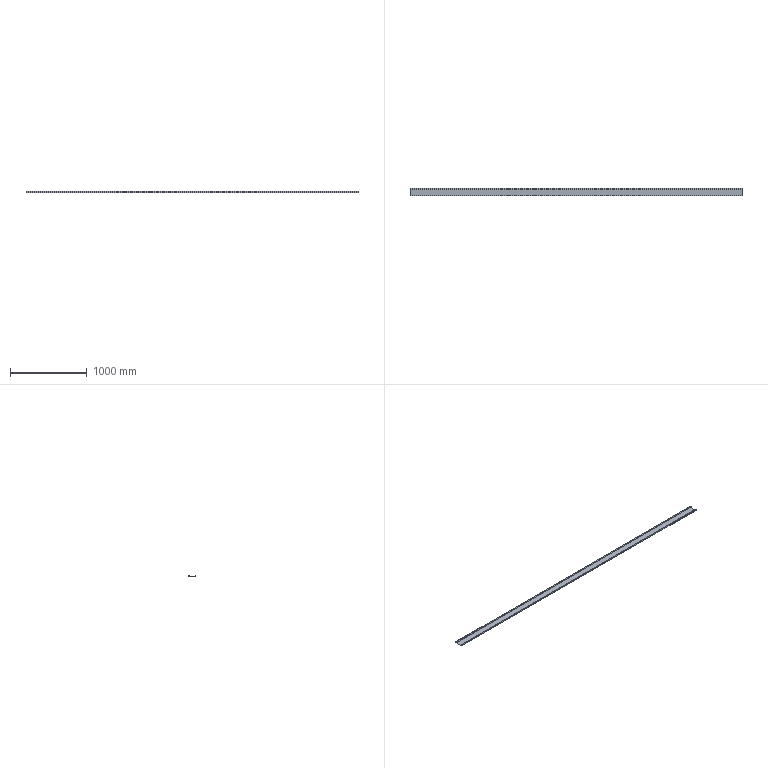Part | STEP file | 电柜护栏4踢脚Plate | 1 solid | 18 faces | box 4333 x 100 x 20 mm | volume 996027 mm3 | plane 12 | cylinder 6 | commonest cylinder face diameters 2 x3 5 x3
STEP:
#1=CARTESIAN_POINT('',(0.,0.,0.));
#2=DIRECTION('',(0.,0.,1.));
#3=DIRECTION('',(1.,0.,0.));
#4=AXIS2_PLACEMENT_3D('',#1,#2,#3);
#5=CARTESIAN_POINT('',(-2166.5,1.5,2.5));
#6=VERTEX_POINT('',#5);
#7=CARTESIAN_POINT('',(-2166.5,1.5,20.));
#8=VERTEX_POINT('',#7);
#9=CARTESIAN_POINT('',(-2166.5,1.5,2.5));
#10=DIRECTION('',(0.,0.,1.));
#11=VECTOR('',#10,1.);
#12=LINE('',#9,#11);
#13=CARTESIAN_POINT('',(2166.5,1.5,2.5));
#14=DIRECTION('',(0.,-1.,0.));
#15=DIRECTION('',(0.,0.,-1.));
#16=AXIS2_PLACEMENT_3D('',#13,#14,#15);
#17=PLANE('',#16);
#18=CARTESIAN_POINT('',(0.,-4333.));
#19=DIRECTION('',(-1.,0.));
#20=VECTOR('',#19,1.);
#21=LINE('',#18,#20);
#22=(GEOMETRIC_REPRESENTATION_CONTEXT(2)PARAMETRIC_REPRESENTATION_CONTEXT()REPRESENTATION_CONTEXT('',''));
#23=DEFINITIONAL_REPRESENTATION('',(#21),#22);
#24=PCURVE('',#17,#23);
#25=CARTESIAN_POINT('',(-2166.5,2.5,2.5));
#26=DIRECTION('',(-1.,0.,0.));
#27=DIRECTION('',(0.,0.,1.));
#28=AXIS2_PLACEMENT_3D('',#25,#26,#27);
#29=PLANE('',#28);
#30=CARTESIAN_POINT('',(0.,-1.));
#31=DIRECTION('',(1.,0.));
#32=VECTOR('',#31,1.);
#33=LINE('',#30,#32);
#34=(GEOMETRIC_REPRESENTATION_CONTEXT(2)PARAMETRIC_REPRESENTATION_CONTEXT()REPRESENTATION_CONTEXT('',''));
#35=DEFINITIONAL_REPRESENTATION('',(#33),#34);
#36=PCURVE('',#29,#35);
#37=SURFACE_CURVE('',#12,(#24,#36),.PCURVE_S1.);
#38=EDGE_CURVE('',#6,#8,#37,.T.);
#39=ORIENTED_EDGE('',*,*,#38,.T.);
#40=CARTESIAN_POINT('',(2166.5,1.5,20.));
#41=VERTEX_POINT('',#40);
#42=CARTESIAN_POINT('',(2166.5,1.5,20.));
#43=DIRECTION('',(-1.,0.,0.));
#44=VECTOR('',#43,1.);
#45=LINE('',#42,#44);
#46=CARTESIAN_POINT('',(-17.5,0.));
#47=DIRECTION('',(0.,-1.));
#48=VECTOR('',#47,1.);
#49=LINE('',#46,#48);
#50=(GEOMETRIC_REPRESENTATION_CONTEXT(2)PARAMETRIC_REPRESENTATION_CONTEXT()REPRESENTATION_CONTEXT('',''));
#51=DEFINITIONAL_REPRESENTATION('',(#49),#50);
#52=PCURVE('',#17,#51);
#53=CARTESIAN_POINT('',(2166.5,0.,20.));
#54=DIRECTION('',(0.,0.,1.));
#55=DIRECTION('',(1.,0.,0.));
#56=AXIS2_PLACEMENT_3D('',#53,#54,#55);
#57=PLANE('',#56);
#58=CARTESIAN_POINT('',(0.,1.5));
#59=DIRECTION('',(-1.,0.));
#60=VECTOR('',#59,1.);
#61=LINE('',#58,#60);
#62=(GEOMETRIC_REPRESENTATION_CONTEXT(2)PARAMETRIC_REPRESENTATION_CONTEXT()REPRESENTATION_CONTEXT('',''));
#63=DEFINITIONAL_REPRESENTATION('',(#61),#62);
#64=PCURVE('',#57,#63);
#65=SURFACE_CURVE('',#45,(#52,#64),.PCURVE_S1.);
#66=EDGE_CURVE('',#41,#8,#65,.T.);
#67=ORIENTED_EDGE('',*,*,#66,.F.);
#68=CARTESIAN_POINT('',(2166.5,1.5,2.5));
#69=VERTEX_POINT('',#68);
#70=CARTESIAN_POINT('',(2166.5,1.5,2.5));
#71=DIRECTION('',(0.,0.,1.));
#72=VECTOR('',#71,1.);
#73=LINE('',#70,#72);
#74=CARTESIAN_POINT('',(0.,0.));
#75=DIRECTION('',(-1.,0.));
#76=VECTOR('',#75,1.);
#77=LINE('',#74,#76);
#78=(GEOMETRIC_REPRESENTATION_CONTEXT(2)PARAMETRIC_REPRESENTATION_CONTEXT()REPRESENTATION_CONTEXT('',''));
#79=DEFINITIONAL_REPRESENTATION('',(#77),#78);
#80=PCURVE('',#17,#79);
#81=CARTESIAN_POINT('',(2166.5,2.5,2.5));
#82=DIRECTION('',(-1.,0.,0.));
#83=DIRECTION('',(0.,0.,1.));
#84=AXIS2_PLACEMENT_3D('',#81,#82,#83);
#85=PLANE('',#84);
#86=CARTESIAN_POINT('',(0.,-1.));
#87=DIRECTION('',(1.,0.));
#88=VECTOR('',#87,1.);
#89=LINE('',#86,#88);
#90=(GEOMETRIC_REPRESENTATION_CONTEXT(2)PARAMETRIC_REPRESENTATION_CONTEXT()REPRESENTATION_CONTEXT('',''));
#91=DEFINITIONAL_REPRESENTATION('',(#89),#90);
#92=PCURVE('',#85,#91);
#93=SURFACE_CURVE('',#73,(#80,#92),.PCURVE_S1.);
#94=EDGE_CURVE('',#69,#41,#93,.T.);
#95=ORIENTED_EDGE('',*,*,#94,.F.);
#96=CARTESIAN_POINT('',(2166.5,1.5,2.5));
#97=DIRECTION('',(-1.,0.,0.));
#98=VECTOR('',#97,1.);
#99=LINE('',#96,#98);
#100=CARTESIAN_POINT('',(0.,0.));
#101=DIRECTION('',(0.,-1.));
#102=VECTOR('',#101,1.);
#103=LINE('',#100,#102);
#104=(GEOMETRIC_REPRESENTATION_CONTEXT(2)PARAMETRIC_REPRESENTATION_CONTEXT()REPRESENTATION_CONTEXT('',''));
#105=DEFINITIONAL_REPRESENTATION('',(#103),#104);
#106=PCURVE('',#17,#105);
#107=CARTESIAN_POINT('',(2166.5,2.5,2.5));
#108=DIRECTION('',(-1.,0.,0.));
#109=DIRECTION('',(0.,0.,1.));
#110=AXIS2_PLACEMENT_3D('',#107,#108,#109);
#111=CYLINDRICAL_SURFACE('',#110,1.);
#112=CARTESIAN_POINT('',(4.712,0.));
#113=DIRECTION('',(0.,1.));
#114=VECTOR('',#113,1.);
#115=LINE('',#112,#114);
#116=(GEOMETRIC_REPRESENTATION_CONTEXT(2)PARAMETRIC_REPRESENTATION_CONTEXT()REPRESENTATION_CONTEXT('',''));
#117=DEFINITIONAL_REPRESENTATION('',(#115),#116);
#118=PCURVE('',#111,#117);
#119=SURFACE_CURVE('',#99,(#106,#118),.PCURVE_S1.);
#120=EDGE_CURVE('',#69,#6,#119,.T.);
#121=ORIENTED_EDGE('',*,*,#120,.T.);
#122=EDGE_LOOP('',(#39,#67,#95,#121));
#123=FACE_BOUND('',#122,.T.);
#124=ADVANCED_FACE('',(#123),#17,.F.);
#125=CARTESIAN_POINT('',(-2166.5,0.,20.));
#126=VERTEX_POINT('',#125);
#127=CARTESIAN_POINT('',(-2166.5,0.,20.));
#128=DIRECTION('',(0.,1.,0.));
#129=VECTOR('',#128,1.);
#130=LINE('',#127,#129);
#131=CARTESIAN_POINT('',(-4333.,0.));
#132=DIRECTION('',(0.,1.));
#133=VECTOR('',#132,1.);
#134=LINE('',#131,#133);
#135=(GEOMETRIC_REPRESENTATION_CONTEXT(2)PARAMETRIC_REPRESENTATION_CONTEXT()REPRESENTATION_CONTEXT('',''));
#136=DEFINITIONAL_REPRESENTATION('',(#134),#135);
#137=PCURVE('',#57,#136);
#138=CARTESIAN_POINT('',(17.5,-2.5));
#139=DIRECTION('',(0.,1.));
#140=VECTOR('',#139,1.);
#141=LINE('',#138,#140);
#142=(GEOMETRIC_REPRESENTATION_CONTEXT(2)PARAMETRIC_REPRESENTATION_CONTEXT()REPRESENTATION_CONTEXT('',''));
#143=DEFINITIONAL_REPRESENTATION('',(#141),#142);
#144=PCURVE('',#29,#143);
#145=SURFACE_CURVE('',#130,(#137,#144),.PCURVE_S1.);
#146=EDGE_CURVE('',#126,#8,#145,.T.);
#147=ORIENTED_EDGE('',*,*,#146,.F.);
#148=CARTESIAN_POINT('',(2166.5,0.,20.));
#149=VERTEX_POINT('',#148);
#150=CARTESIAN_POINT('',(2166.5,0.,20.));
#151=DIRECTION('',(-1.,0.,0.));
#152=VECTOR('',#151,1.);
#153=LINE('',#150,#152);
#154=CARTESIAN_POINT('',(0.,0.));
#155=DIRECTION('',(-1.,0.));
#156=VECTOR('',#155,1.);
#157=LINE('',#154,#156);
#158=(GEOMETRIC_REPRESENTATION_CONTEXT(2)PARAMETRIC_REPRESENTATION_CONTEXT()REPRESENTATION_CONTEXT('',''));
#159=DEFINITIONAL_REPRESENTATION('',(#157),#158);
#160=PCURVE('',#57,#159);
#161=CARTESIAN_POINT('',(2166.5,0.,2.5));
#162=DIRECTION('',(0.,-1.,0.));
#163=DIRECTION('',(0.,0.,-1.));
#164=AXIS2_PLACEMENT_3D('',#161,#162,#163);
#165=PLANE('',#164);
#166=CARTESIAN_POINT('',(-17.5,0.));
#167=DIRECTION('',(0.,-1.));
#168=VECTOR('',#167,1.);
#169=LINE('',#166,#168);
#170=(GEOMETRIC_REPRESENTATION_CONTEXT(2)PARAMETRIC_REPRESENTATION_CONTEXT()REPRESENTATION_CONTEXT('',''));
#171=DEFINITIONAL_REPRESENTATION('',(#169),#170);
#172=PCURVE('',#165,#171);
#173=SURFACE_CURVE('',#153,(#160,#172),.PCURVE_S1.);
#174=EDGE_CURVE('',#149,#126,#173,.T.);
#175=ORIENTED_EDGE('',*,*,#174,.F.);
#176=CARTESIAN_POINT('',(2166.5,0.,20.));
#177=DIRECTION('',(0.,1.,0.));
#178=VECTOR('',#177,1.);
#179=LINE('',#176,#178);
#180=CARTESIAN_POINT('',(0.,0.));
#181=DIRECTION('',(0.,1.));
#182=VECTOR('',#181,1.);
#183=LINE('',#180,#182);
#184=(GEOMETRIC_REPRESENTATION_CONTEXT(2)PARAMETRIC_REPRESENTATION_CONTEXT()REPRESENTATION_CONTEXT('',''));
#185=DEFINITIONAL_REPRESENTATION('',(#183),#184);
#186=PCURVE('',#57,#185);
#187=CARTESIAN_POINT('',(17.5,-2.5));
#188=DIRECTION('',(0.,1.));
#189=VECTOR('',#188,1.);
#190=LINE('',#187,#189);
#191=(GEOMETRIC_REPRESENTATION_CONTEXT(2)PARAMETRIC_REPRESENTATION_CONTEXT()REPRESENTATION_CONTEXT('',''));
#192=DEFINITIONAL_REPRESENTATION('',(#190),#191);
#193=PCURVE('',#85,#192);
#194=SURFACE_CURVE('',#179,(#186,#193),.PCURVE_S1.);
#195=EDGE_CURVE('',#149,#41,#194,.T.);
#196=ORIENTED_EDGE('',*,*,#195,.T.);
#197=ORIENTED_EDGE('',*,*,#66,.T.);
#198=EDGE_LOOP('',(#147,#175,#196,#197));
#199=FACE_BOUND('',#198,.T.);
#200=ADVANCED_FACE('',(#199),#57,.T.);
#201=CARTESIAN_POINT('',(-2166.5,0.,2.5));
#202=VERTEX_POINT('',#201);
#203=CARTESIAN_POINT('',(-2166.5,0.,2.5));
#204=DIRECTION('',(0.,0.,1.));
#205=VECTOR('',#204,1.);
#206=LINE('',#203,#205);
#207=CARTESIAN_POINT('',(0.,-4333.));
#208=DIRECTION('',(-1.,0.));
#209=VECTOR('',#208,1.);
#210=LINE('',#207,#209);
#211=(GEOMETRIC_REPRESENTATION_CONTEXT(2)PARAMETRIC_REPRESENTATION_CONTEXT()REPRESENTATION_CONTEXT('',''));
#212=DEFINITIONAL_REPRESENTATION('',(#210),#211);
#213=PCURVE('',#165,#212);
#214=CARTESIAN_POINT('',(0.,-2.5));
#215=DIRECTION('',(1.,0.));
#216=VECTOR('',#215,1.);
#217=LINE('',#214,#216);
#218=(GEOMETRIC_REPRESENTATION_CONTEXT(2)PARAMETRIC_REPRESENTATION_CONTEXT()REPRESENTATION_CONTEXT('',''));
#219=DEFINITIONAL_REPRESENTATION('',(#217),#218);
#220=PCURVE('',#29,#219);
#221=SURFACE_CURVE('',#206,(#213,#220),.PCURVE_S1.);
#222=EDGE_CURVE('',#202,#126,#221,.T.);
#223=ORIENTED_EDGE('',*,*,#222,.F.);
#224=CARTESIAN_POINT('',(2166.5,0.,2.5));
#225=VERTEX_POINT('',#224);
#226=CARTESIAN_POINT('',(2166.5,0.,2.5));
#227=DIRECTION('',(-1.,0.,0.));
#228=VECTOR('',#227,1.);
#229=LINE('',#226,#228);
#230=CARTESIAN_POINT('',(0.,0.));
#231=DIRECTION('',(0.,-1.));
#232=VECTOR('',#231,1.);
#233=LINE('',#230,#232);
#234=(GEOMETRIC_REPRESENTATION_CONTEXT(2)PARAMETRIC_REPRESENTATION_CONTEXT()REPRESENTATION_CONTEXT('',''));
#235=DEFINITIONAL_REPRESENTATION('',(#233),#234);
#236=PCURVE('',#165,#235);
#237=CARTESIAN_POINT('',(2166.5,2.5,2.5));
#238=DIRECTION('',(-1.,0.,0.));
#239=DIRECTION('',(0.,0.,1.));
#240=AXIS2_PLACEMENT_3D('',#237,#238,#239);
#241=CYLINDRICAL_SURFACE('',#240,2.5);
#242=CARTESIAN_POINT('',(4.712,0.));
#243=DIRECTION('',(0.,1.));
#244=VECTOR('',#243,1.);
#245=LINE('',#242,#244);
#246=(GEOMETRIC_REPRESENTATION_CONTEXT(2)PARAMETRIC_REPRESENTATION_CONTEXT()REPRESENTATION_CONTEXT('',''));
#247=DEFINITIONAL_REPRESENTATION('',(#245),#246);
#248=PCURVE('',#241,#247);
#249=SURFACE_CURVE('',#229,(#236,#248),.PCURVE_S1.);
#250=EDGE_CURVE('',#225,#202,#249,.T.);
#251=ORIENTED_EDGE('',*,*,#250,.F.);
#252=CARTESIAN_POINT('',(2166.5,0.,2.5));
#253=DIRECTION('',(0.,0.,1.));
#254=VECTOR('',#253,1.);
#255=LINE('',#252,#254);
#256=CARTESIAN_POINT('',(0.,0.));
#257=DIRECTION('',(-1.,0.));
#258=VECTOR('',#257,1.);
#259=LINE('',#256,#258);
#260=(GEOMETRIC_REPRESENTATION_CONTEXT(2)PARAMETRIC_REPRESENTATION_CONTEXT()REPRESENTATION_CONTEXT('',''));
#261=DEFINITIONAL_REPRESENTATION('',(#259),#260);
#262=PCURVE('',#165,#261);
#263=CARTESIAN_POINT('',(0.,-2.5));
#264=DIRECTION('',(1.,0.));
#265=VECTOR('',#264,1.);
#266=LINE('',#263,#265);
#267=(GEOMETRIC_REPRESENTATION_CONTEXT(2)PARAMETRIC_REPRESENTATION_CONTEXT()REPRESENTATION_CONTEXT('',''));
#268=DEFINITIONAL_REPRESENTATION('',(#266),#267);
#269=PCURVE('',#85,#268);
#270=SURFACE_CURVE('',#255,(#262,#269),.PCURVE_S1.);
#271=EDGE_CURVE('',#225,#149,#270,.T.);
#272=ORIENTED_EDGE('',*,*,#271,.T.);
#273=ORIENTED_EDGE('',*,*,#174,.T.);
#274=EDGE_LOOP('',(#223,#251,#272,#273));
#275=FACE_BOUND('',#274,.T.);
#276=ADVANCED_FACE('',(#275),#165,.T.);
#277=CARTESIAN_POINT('',(-2166.5,2.5,0.));
#278=VERTEX_POINT('',#277);
#279=CARTESIAN_POINT('',(-2166.5,2.5,2.5));
#280=DIRECTION('',(-1.,0.,0.));
#281=DIRECTION('',(0.,0.,1.));
#282=AXIS2_PLACEMENT_3D('',#279,#280,#281);
#283=CIRCLE('',#282,2.5);
#284=CARTESIAN_POINT('',(0.,4333.));
#285=DIRECTION('',(1.,0.));
#286=VECTOR('',#285,1.);
#287=LINE('',#284,#286);
#288=(GEOMETRIC_REPRESENTATION_CONTEXT(2)PARAMETRIC_REPRESENTATION_CONTEXT()REPRESENTATION_CONTEXT('',''));
#289=DEFINITIONAL_REPRESENTATION('',(#287),#288);
#290=PCURVE('',#241,#289);
#291=CARTESIAN_POINT('',(0.,0.));
#292=DIRECTION('',(1.,0.));
#293=AXIS2_PLACEMENT_2D('',#291,#292);
#294=CIRCLE('',#293,2.5);
#295=(GEOMETRIC_REPRESENTATION_CONTEXT(2)PARAMETRIC_REPRESENTATION_CONTEXT()REPRESENTATION_CONTEXT('',''));
#296=DEFINITIONAL_REPRESENTATION('',(#294),#295);
#297=PCURVE('',#29,#296);
#298=SURFACE_CURVE('',#283,(#290,#297),.PCURVE_S1.);
#299=EDGE_CURVE('',#278,#202,#298,.T.);
#300=ORIENTED_EDGE('',*,*,#299,.F.);
#301=CARTESIAN_POINT('',(2166.5,2.5,0.));
#302=VERTEX_POINT('',#301);
#303=CARTESIAN_POINT('',(2166.5,2.5,0.));
#304=DIRECTION('',(-1.,0.,0.));
#305=VECTOR('',#304,1.);
#306=LINE('',#303,#305);
#307=CARTESIAN_POINT('',(3.142,0.));
#308=DIRECTION('',(0.,1.));
#309=VECTOR('',#308,1.);
#310=LINE('',#307,#309);
#311=(GEOMETRIC_REPRESENTATION_CONTEXT(2)PARAMETRIC_REPRESENTATION_CONTEXT()REPRESENTATION_CONTEXT('',''));
#312=DEFINITIONAL_REPRESENTATION('',(#310),#311);
#313=PCURVE('',#241,#312);
#314=CARTESIAN_POINT('',(2166.5,2.5,0.));
#315=DIRECTION('',(0.,0.,-1.));
#316=DIRECTION('',(-1.,0.,0.));
#317=AXIS2_PLACEMENT_3D('',#314,#315,#316);
#318=PLANE('',#317);
#319=CARTESIAN_POINT('',(0.,0.));
#320=DIRECTION('',(1.,0.));
#321=VECTOR('',#320,1.);
#322=LINE('',#319,#321);
#323=(GEOMETRIC_REPRESENTATION_CONTEXT(2)PARAMETRIC_REPRESENTATION_CONTEXT()REPRESENTATION_CONTEXT('',''));
#324=DEFINITIONAL_REPRESENTATION('',(#322),#323);
#325=PCURVE('',#318,#324);
#326=SURFACE_CURVE('',#306,(#313,#325),.PCURVE_S1.);
#327=EDGE_CURVE('',#302,#278,#326,.T.);
#328=ORIENTED_EDGE('',*,*,#327,.F.);
#329=CARTESIAN_POINT('',(2166.5,2.5,2.5));
#330=DIRECTION('',(-1.,0.,0.));
#331=DIRECTION('',(0.,0.,1.));
#332=AXIS2_PLACEMENT_3D('',#329,#330,#331);
#333=CIRCLE('',#332,2.5);
#334=CARTESIAN_POINT('',(0.,0.));
#335=DIRECTION('',(1.,0.));
#336=VECTOR('',#335,1.);
#337=LINE('',#334,#336);
#338=(GEOMETRIC_REPRESENTATION_CONTEXT(2)PARAMETRIC_REPRESENTATION_CONTEXT()REPRESENTATION_CONTEXT('',''));
#339=DEFINITIONAL_REPRESENTATION('',(#337),#338);
#340=PCURVE('',#241,#339);
#341=CARTESIAN_POINT('',(0.,0.));
#342=DIRECTION('',(1.,0.));
#343=AXIS2_PLACEMENT_2D('',#341,#342);
#344=CIRCLE('',#343,2.5);
#345=(GEOMETRIC_REPRESENTATION_CONTEXT(2)PARAMETRIC_REPRESENTATION_CONTEXT()REPRESENTATION_CONTEXT('',''));
#346=DEFINITIONAL_REPRESENTATION('',(#344),#345);
#347=PCURVE('',#85,#346);
#348=SURFACE_CURVE('',#333,(#340,#347),.PCURVE_S1.);
#349=EDGE_CURVE('',#302,#225,#348,.T.);
#350=ORIENTED_EDGE('',*,*,#349,.T.);
#351=ORIENTED_EDGE('',*,*,#250,.T.);
#352=EDGE_LOOP('',(#300,#328,#350,#351));
#353=FACE_BOUND('',#352,.T.);
#354=ADVANCED_FACE('',(#353),#241,.T.);
#355=CARTESIAN_POINT('',(-2166.5,97.5,0.));
#356=VERTEX_POINT('',#355);
#357=CARTESIAN_POINT('',(-2166.5,2.5,0.));
#358=DIRECTION('',(0.,-1.,0.));
#359=VECTOR('',#358,1.);
#360=LINE('',#357,#359);
#361=CARTESIAN_POINT('',(4333.,0.));
#362=DIRECTION('',(0.,-1.));
#363=VECTOR('',#362,1.);
#364=LINE('',#361,#363);
#365=(GEOMETRIC_REPRESENTATION_CONTEXT(2)PARAMETRIC_REPRESENTATION_CONTEXT()REPRESENTATION_CONTEXT('',''));
#366=DEFINITIONAL_REPRESENTATION('',(#364),#365);
#367=PCURVE('',#318,#366);
#368=CARTESIAN_POINT('',(-2.5,0.));
#369=DIRECTION('',(0.,-1.));
#370=VECTOR('',#369,1.);
#371=LINE('',#368,#370);
#372=(GEOMETRIC_REPRESENTATION_CONTEXT(2)PARAMETRIC_REPRESENTATION_CONTEXT()REPRESENTATION_CONTEXT('',''));
#373=DEFINITIONAL_REPRESENTATION('',(#371),#372);
#374=PCURVE('',#29,#373);
#375=SURFACE_CURVE('',#360,(#367,#374),.PCURVE_S1.);
#376=EDGE_CURVE('',#356,#278,#375,.T.);
#377=ORIENTED_EDGE('',*,*,#376,.F.);
#378=CARTESIAN_POINT('',(2166.5,97.5,0.));
#379=VERTEX_POINT('',#378);
#380=CARTESIAN_POINT('',(2166.5,97.5,0.));
#381=DIRECTION('',(-1.,0.,0.));
#382=VECTOR('',#381,1.);
#383=LINE('',#380,#382);
#384=CARTESIAN_POINT('',(0.,95.));
#385=DIRECTION('',(1.,0.));
#386=VECTOR('',#385,1.);
#387=LINE('',#384,#386);
#388=(GEOMETRIC_REPRESENTATION_CONTEXT(2)PARAMETRIC_REPRESENTATION_CONTEXT()REPRESENTATION_CONTEXT('',''));
#389=DEFINITIONAL_REPRESENTATION('',(#387),#388);
#390=PCURVE('',#318,#389);
#391=CARTESIAN_POINT('',(2166.5,97.5,2.5));
#392=DIRECTION('',(-1.,0.,0.));
#393=DIRECTION('',(0.,0.,1.));
#394=AXIS2_PLACEMENT_3D('',#391,#392,#393);
#395=CYLINDRICAL_SURFACE('',#394,2.5);
#396=CARTESIAN_POINT('',(3.142,0.));
#397=DIRECTION('',(0.,1.));
#398=VECTOR('',#397,1.);
#399=LINE('',#396,#398);
#400=(GEOMETRIC_REPRESENTATION_CONTEXT(2)PARAMETRIC_REPRESENTATION_CONTEXT()REPRESENTATION_CONTEXT('',''));
#401=DEFINITIONAL_REPRESENTATION('',(#399),#400);
#402=PCURVE('',#395,#401);
#403=SURFACE_CURVE('',#383,(#390,#402),.PCURVE_S1.);
#404=EDGE_CURVE('',#379,#356,#403,.T.);
#405=ORIENTED_EDGE('',*,*,#404,.F.);
#406=CARTESIAN_POINT('',(2166.5,2.5,0.));
#407=DIRECTION('',(0.,-1.,0.));
#408=VECTOR('',#407,1.);
#409=LINE('',#406,#408);
#410=CARTESIAN_POINT('',(0.,0.));
#411=DIRECTION('',(0.,-1.));
#412=VECTOR('',#411,1.);
#413=LINE('',#410,#412);
#414=(GEOMETRIC_REPRESENTATION_CONTEXT(2)PARAMETRIC_REPRESENTATION_CONTEXT()REPRESENTATION_CONTEXT('',''));
#415=DEFINITIONAL_REPRESENTATION('',(#413),#414);
#416=PCURVE('',#318,#415);
#417=CARTESIAN_POINT('',(-2.5,0.));
#418=DIRECTION('',(0.,-1.));
#419=VECTOR('',#418,1.);
#420=LINE('',#417,#419);
#421=(GEOMETRIC_REPRESENTATION_CONTEXT(2)PARAMETRIC_REPRESENTATION_CONTEXT()REPRESENTATION_CONTEXT('',''));
#422=DEFINITIONAL_REPRESENTATION('',(#420),#421);
#423=PCURVE('',#85,#422);
#424=SURFACE_CURVE('',#409,(#416,#423),.PCURVE_S1.);
#425=EDGE_CURVE('',#379,#302,#424,.T.);
#426=ORIENTED_EDGE('',*,*,#425,.T.);
#427=ORIENTED_EDGE('',*,*,#327,.T.);
#428=EDGE_LOOP('',(#377,#405,#426,#427));
#429=FACE_BOUND('',#428,.T.);
#430=ADVANCED_FACE('',(#429),#318,.T.);
#431=CARTESIAN_POINT('',(-2166.5,100.,2.5));
#432=VERTEX_POINT('',#431);
#433=CARTESIAN_POINT('',(-2166.5,97.5,2.5));
#434=DIRECTION('',(-1.,0.,0.));
#435=DIRECTION('',(0.,0.,-1.));
#436=AXIS2_PLACEMENT_3D('',#433,#434,#435);
#437=CIRCLE('',#436,2.5);
#438=CARTESIAN_POINT('',(-3.142,4333.));
#439=DIRECTION('',(1.,0.));
#440=VECTOR('',#439,1.);
#441=LINE('',#438,#440);
#442=(GEOMETRIC_REPRESENTATION_CONTEXT(2)PARAMETRIC_REPRESENTATION_CONTEXT()REPRESENTATION_CONTEXT('',''));
#443=DEFINITIONAL_REPRESENTATION('',(#441),#442);
#444=PCURVE('',#395,#443);
#445=CARTESIAN_POINT('',(0.,95.));
#446=DIRECTION('',(-1.,0.));
#447=AXIS2_PLACEMENT_2D('',#445,#446);
#448=CIRCLE('',#447,2.5);
#449=(GEOMETRIC_REPRESENTATION_CONTEXT(2)PARAMETRIC_REPRESENTATION_CONTEXT()REPRESENTATION_CONTEXT('',''));
#450=DEFINITIONAL_REPRESENTATION('',(#448),#449);
#451=PCURVE('',#29,#450);
#452=SURFACE_CURVE('',#437,(#444,#451),.PCURVE_S1.);
#453=EDGE_CURVE('',#432,#356,#452,.T.);
#454=ORIENTED_EDGE('',*,*,#453,.F.);
#455=CARTESIAN_POINT('',(2166.5,100.,2.5));
#456=VERTEX_POINT('',#455);
#457=CARTESIAN_POINT('',(2166.5,100.,2.5));
#458=DIRECTION('',(-1.,0.,0.));
#459=VECTOR('',#458,1.);
#460=LINE('',#457,#459);
#461=CARTESIAN_POINT('',(1.571,0.));
#462=DIRECTION('',(0.,1.));
#463=VECTOR('',#462,1.);
#464=LINE('',#461,#463);
#465=(GEOMETRIC_REPRESENTATION_CONTEXT(2)PARAMETRIC_REPRESENTATION_CONTEXT()REPRESENTATION_CONTEXT('',''));
#466=DEFINITIONAL_REPRESENTATION('',(#464),#465);
#467=PCURVE('',#395,#466);
#468=CARTESIAN_POINT('',(2166.5,100.,2.5));
#469=DIRECTION('',(0.,1.,0.));
#470=DIRECTION('',(0.,0.,1.));
#471=AXIS2_PLACEMENT_3D('',#468,#469,#470);
#472=PLANE('',#471);
#473=CARTESIAN_POINT('',(0.,0.));
#474=DIRECTION('',(0.,-1.));
#475=VECTOR('',#474,1.);
#476=LINE('',#473,#475);
#477=(GEOMETRIC_REPRESENTATION_CONTEXT(2)PARAMETRIC_REPRESENTATION_CONTEXT()REPRESENTATION_CONTEXT('',''));
#478=DEFINITIONAL_REPRESENTATION('',(#476),#477);
#479=PCURVE('',#472,#478);
#480=SURFACE_CURVE('',#460,(#467,#479),.PCURVE_S1.);
#481=EDGE_CURVE('',#456,#432,#480,.T.);
#482=ORIENTED_EDGE('',*,*,#481,.F.);
#483=CARTESIAN_POINT('',(2166.5,97.5,2.5));
#484=DIRECTION('',(-1.,0.,0.));
#485=DIRECTION('',(0.,0.,-1.));
#486=AXIS2_PLACEMENT_3D('',#483,#484,#485);
#487=CIRCLE('',#486,2.5);
#488=CARTESIAN_POINT('',(-3.142,0.));
#489=DIRECTION('',(1.,0.));
#490=VECTOR('',#489,1.);
#491=LINE('',#488,#490);
#492=(GEOMETRIC_REPRESENTATION_CONTEXT(2)PARAMETRIC_REPRESENTATION_CONTEXT()REPRESENTATION_CONTEXT('',''));
#493=DEFINITIONAL_REPRESENTATION('',(#491),#492);
#494=PCURVE('',#395,#493);
#495=CARTESIAN_POINT('',(0.,95.));
#496=DIRECTION('',(-1.,0.));
#497=AXIS2_PLACEMENT_2D('',#495,#496);
#498=CIRCLE('',#497,2.5);
#499=(GEOMETRIC_REPRESENTATION_CONTEXT(2)PARAMETRIC_REPRESENTATION_CONTEXT()REPRESENTATION_CONTEXT('',''));
#500=DEFINITIONAL_REPRESENTATION('',(#498),#499);
#501=PCURVE('',#85,#500);
#502=SURFACE_CURVE('',#487,(#494,#501),.PCURVE_S1.);
#503=EDGE_CURVE('',#456,#379,#502,.T.);
#504=ORIENTED_EDGE('',*,*,#503,.T.);
#505=ORIENTED_EDGE('',*,*,#404,.T.);
#506=EDGE_LOOP('',(#454,#482,#504,#505));
#507=FACE_BOUND('',#506,.T.);
#508=ADVANCED_FACE('',(#507),#395,.T.);
#509=CARTESIAN_POINT('',(-2166.5,100.,17.5));
#510=VERTEX_POINT('',#509);
#511=CARTESIAN_POINT('',(-2166.5,100.,2.5));
#512=DIRECTION('',(0.,0.,-1.));
#513=VECTOR('',#512,1.);
#514=LINE('',#511,#513);
#515=CARTESIAN_POINT('',(0.,-4333.));
#516=DIRECTION('',(-1.,0.));
#517=VECTOR('',#516,1.);
#518=LINE('',#515,#517);
#519=(GEOMETRIC_REPRESENTATION_CONTEXT(2)PARAMETRIC_REPRESENTATION_CONTEXT()REPRESENTATION_CONTEXT('',''));
#520=DEFINITIONAL_REPRESENTATION('',(#518),#519);
#521=PCURVE('',#472,#520);
#522=CARTESIAN_POINT('',(0.,97.5));
#523=DIRECTION('',(-1.,0.));
#524=VECTOR('',#523,1.);
#525=LINE('',#522,#524);
#526=(GEOMETRIC_REPRESENTATION_CONTEXT(2)PARAMETRIC_REPRESENTATION_CONTEXT()REPRESENTATION_CONTEXT('',''));
#527=DEFINITIONAL_REPRESENTATION('',(#525),#526);
#528=PCURVE('',#29,#527);
#529=SURFACE_CURVE('',#514,(#521,#528),.PCURVE_S1.);
#530=EDGE_CURVE('',#510,#432,#529,.T.);
#531=ORIENTED_EDGE('',*,*,#530,.F.);
#532=CARTESIAN_POINT('',(2166.5,100.,17.5));
#533=VERTEX_POINT('',#532);
#534=CARTESIAN_POINT('',(2166.5,100.,17.5));
#535=DIRECTION('',(-1.,0.,0.));
#536=VECTOR('',#535,1.);
#537=LINE('',#534,#536);
#538=CARTESIAN_POINT('',(15.,0.));
#539=DIRECTION('',(0.,-1.));
#540=VECTOR('',#539,1.);
#541=LINE('',#538,#540);
#542=(GEOMETRIC_REPRESENTATION_CONTEXT(2)PARAMETRIC_REPRESENTATION_CONTEXT()REPRESENTATION_CONTEXT('',''));
#543=DEFINITIONAL_REPRESENTATION('',(#541),#542);
#544=PCURVE('',#472,#543);
#545=CARTESIAN_POINT('',(2166.5,97.5,17.5));
#546=DIRECTION('',(-1.,0.,0.));
#547=DIRECTION('',(0.,0.,1.));
#548=AXIS2_PLACEMENT_3D('',#545,#546,#547);
#549=CYLINDRICAL_SURFACE('',#548,2.5);
#550=CARTESIAN_POINT('',(1.571,0.));
#551=DIRECTION('',(0.,1.));
#552=VECTOR('',#551,1.);
#553=LINE('',#550,#552);
#554=(GEOMETRIC_REPRESENTATION_CONTEXT(2)PARAMETRIC_REPRESENTATION_CONTEXT()REPRESENTATION_CONTEXT('',''));
#555=DEFINITIONAL_REPRESENTATION('',(#553),#554);
#556=PCURVE('',#549,#555);
#557=SURFACE_CURVE('',#537,(#544,#556),.PCURVE_S1.);
#558=EDGE_CURVE('',#533,#510,#557,.T.);
#559=ORIENTED_EDGE('',*,*,#558,.F.);
#560=CARTESIAN_POINT('',(2166.5,100.,2.5));
#561=DIRECTION('',(0.,0.,-1.));
#562=VECTOR('',#561,1.);
#563=LINE('',#560,#562);
#564=CARTESIAN_POINT('',(0.,0.));
#565=DIRECTION('',(-1.,0.));
#566=VECTOR('',#565,1.);
#567=LINE('',#564,#566);
#568=(GEOMETRIC_REPRESENTATION_CONTEXT(2)PARAMETRIC_REPRESENTATION_CONTEXT()REPRESENTATION_CONTEXT('',''));
#569=DEFINITIONAL_REPRESENTATION('',(#567),#568);
#570=PCURVE('',#472,#569);
#571=CARTESIAN_POINT('',(0.,97.5));
#572=DIRECTION('',(-1.,0.));
#573=VECTOR('',#572,1.);
#574=LINE('',#571,#573);
#575=(GEOMETRIC_REPRESENTATION_CONTEXT(2)PARAMETRIC_REPRESENTATION_CONTEXT()REPRESENTATION_CONTEXT('',''));
#576=DEFINITIONAL_REPRESENTATION('',(#574),#575);
#577=PCURVE('',#85,#576);
#578=SURFACE_CURVE('',#563,(#570,#577),.PCURVE_S1.);
#579=EDGE_CURVE('',#533,#456,#578,.T.);
#580=ORIENTED_EDGE('',*,*,#579,.T.);
#581=ORIENTED_EDGE('',*,*,#481,.T.);
#582=EDGE_LOOP('',(#531,#559,#580,#581));
#583=FACE_BOUND('',#582,.T.);
#584=ADVANCED_FACE('',(#583),#472,.T.);
#585=CARTESIAN_POINT('',(-2166.5,97.5,20.));
#586=VERTEX_POINT('',#585);
#587=CARTESIAN_POINT('',(-2166.5,97.5,17.5));
#588=DIRECTION('',(-1.,0.,0.));
#589=DIRECTION('',(0.,0.,-1.));
#590=AXIS2_PLACEMENT_3D('',#587,#588,#589);
#591=CIRCLE('',#590,2.5);
#592=CARTESIAN_POINT('',(-3.142,4333.));
#593=DIRECTION('',(1.,0.));
#594=VECTOR('',#593,1.);
#595=LINE('',#592,#594);
#596=(GEOMETRIC_REPRESENTATION_CONTEXT(2)PARAMETRIC_REPRESENTATION_CONTEXT()REPRESENTATION_CONTEXT('',''));
#597=DEFINITIONAL_REPRESENTATION('',(#595),#596);
#598=PCURVE('',#549,#597);
#599=CARTESIAN_POINT('',(15.,95.));
#600=DIRECTION('',(-1.,0.));
#601=AXIS2_PLACEMENT_2D('',#599,#600);
#602=CIRCLE('',#601,2.5);
#603=(GEOMETRIC_REPRESENTATION_CONTEXT(2)PARAMETRIC_REPRESENTATION_CONTEXT()REPRESENTATION_CONTEXT('',''));
#604=DEFINITIONAL_REPRESENTATION('',(#602),#603);
#605=PCURVE('',#29,#604);
#606=SURFACE_CURVE('',#591,(#598,#605),.PCURVE_S1.);
#607=EDGE_CURVE('',#586,#510,#606,.T.);
#608=ORIENTED_EDGE('',*,*,#607,.F.);
#609=CARTESIAN_POINT('',(2166.5,97.5,20.));
#610=VERTEX_POINT('',#609);
#611=CARTESIAN_POINT('',(2166.5,97.5,20.));
#612=DIRECTION('',(-1.,0.,0.));
#613=VECTOR('',#612,1.);
#614=LINE('',#611,#613);
#615=CARTESIAN_POINT('',(0.,0.));
#616=DIRECTION('',(0.,1.));
#617=VECTOR('',#616,1.);
#618=LINE('',#615,#617);
#619=(GEOMETRIC_REPRESENTATION_CONTEXT(2)PARAMETRIC_REPRESENTATION_CONTEXT()REPRESENTATION_CONTEXT('',''));
#620=DEFINITIONAL_REPRESENTATION('',(#618),#619);
#621=PCURVE('',#549,#620);
#622=CARTESIAN_POINT('',(2166.5,97.5,20.));
#623=DIRECTION('',(0.,0.,1.));
#624=DIRECTION('',(1.,0.,0.));
#625=AXIS2_PLACEMENT_3D('',#622,#623,#624);
#626=PLANE('',#625);
#627=CARTESIAN_POINT('',(0.,0.));
#628=DIRECTION('',(-1.,0.));
#629=VECTOR('',#628,1.);
#630=LINE('',#627,#629);
#631=(GEOMETRIC_REPRESENTATION_CONTEXT(2)PARAMETRIC_REPRESENTATION_CONTEXT()REPRESENTATION_CONTEXT('',''));
#632=DEFINITIONAL_REPRESENTATION('',(#630),#631);
#633=PCURVE('',#626,#632);
#634=SURFACE_CURVE('',#614,(#621,#633),.PCURVE_S1.);
#635=EDGE_CURVE('',#610,#586,#634,.T.);
#636=ORIENTED_EDGE('',*,*,#635,.F.);
#637=CARTESIAN_POINT('',(2166.5,97.5,17.5));
#638=DIRECTION('',(-1.,0.,0.));
#639=DIRECTION('',(0.,0.,-1.));
#640=AXIS2_PLACEMENT_3D('',#637,#638,#639);
#641=CIRCLE('',#640,2.5);
#642=CARTESIAN_POINT('',(-3.142,0.));
#643=DIRECTION('',(1.,0.));
#644=VECTOR('',#643,1.);
#645=LINE('',#642,#644);
#646=(GEOMETRIC_REPRESENTATION_CONTEXT(2)PARAMETRIC_REPRESENTATION_CONTEXT()REPRESENTATION_CONTEXT('',''));
#647=DEFINITIONAL_REPRESENTATION('',(#645),#646);
#648=PCURVE('',#549,#647);
#649=CARTESIAN_POINT('',(15.,95.));
#650=DIRECTION('',(-1.,0.));
#651=AXIS2_PLACEMENT_2D('',#649,#650);
#652=CIRCLE('',#651,2.5);
#653=(GEOMETRIC_REPRESENTATION_CONTEXT(2)PARAMETRIC_REPRESENTATION_CONTEXT()REPRESENTATION_CONTEXT('',''));
#654=DEFINITIONAL_REPRESENTATION('',(#652),#653);
#655=PCURVE('',#85,#654);
#656=SURFACE_CURVE('',#641,(#648,#655),.PCURVE_S1.);
#657=EDGE_CURVE('',#610,#533,#656,.T.);
#658=ORIENTED_EDGE('',*,*,#657,.T.);
#659=ORIENTED_EDGE('',*,*,#558,.T.);
#660=EDGE_LOOP('',(#608,#636,#658,#659));
#661=FACE_BOUND('',#660,.T.);
#662=ADVANCED_FACE('',(#661),#549,.T.);
#663=CARTESIAN_POINT('',(-2166.5,80.,20.));
#664=VERTEX_POINT('',#663);
#665=CARTESIAN_POINT('',(-2166.5,97.5,20.));
#666=DIRECTION('',(0.,1.,0.));
#667=VECTOR('',#666,1.);
#668=LINE('',#665,#667);
#669=CARTESIAN_POINT('',(-4333.,0.));
#670=DIRECTION('',(0.,1.));
#671=VECTOR('',#670,1.);
#672=LINE('',#669,#671);
#673=(GEOMETRIC_REPRESENTATION_CONTEXT(2)PARAMETRIC_REPRESENTATION_CONTEXT()REPRESENTATION_CONTEXT('',''));
#674=DEFINITIONAL_REPRESENTATION('',(#672),#673);
#675=PCURVE('',#626,#674);
#676=CARTESIAN_POINT('',(17.5,95.));
#677=DIRECTION('',(0.,1.));
#678=VECTOR('',#677,1.);
#679=LINE('',#676,#678);
#680=(GEOMETRIC_REPRESENTATION_CONTEXT(2)PARAMETRIC_REPRESENTATION_CONTEXT()REPRESENTATION_CONTEXT('',''));
#681=DEFINITIONAL_REPRESENTATION('',(#679),#680);
#682=PCURVE('',#29,#681);
#683=SURFACE_CURVE('',#668,(#675,#682),.PCURVE_S1.);
#684=EDGE_CURVE('',#664,#586,#683,.T.);
#685=ORIENTED_EDGE('',*,*,#684,.F.);
#686=CARTESIAN_POINT('',(2166.5,80.,20.));
#687=VERTEX_POINT('',#686);
#688=CARTESIAN_POINT('',(2166.5,80.,20.));
#689=DIRECTION('',(-1.,0.,0.));
#690=VECTOR('',#689,1.);
#691=LINE('',#688,#690);
#692=CARTESIAN_POINT('',(0.,-17.5));
#693=DIRECTION('',(-1.,0.));
#694=VECTOR('',#693,1.);
#695=LINE('',#692,#694);
#696=(GEOMETRIC_REPRESENTATION_CONTEXT(2)PARAMETRIC_REPRESENTATION_CONTEXT()REPRESENTATION_CONTEXT('',''));
#697=DEFINITIONAL_REPRESENTATION('',(#695),#696);
#698=PCURVE('',#626,#697);
#699=CARTESIAN_POINT('',(2166.5,80.,18.5));
#700=DIRECTION('',(0.,-1.,0.));
#701=DIRECTION('',(0.,0.,-1.));
#702=AXIS2_PLACEMENT_3D('',#699,#700,#701);
#703=PLANE('',#702);
#704=CARTESIAN_POINT('',(-1.5,0.));
#705=DIRECTION('',(0.,-1.));
#706=VECTOR('',#705,1.);
#707=LINE('',#704,#706);
#708=(GEOMETRIC_REPRESENTATION_CONTEXT(2)PARAMETRIC_REPRESENTATION_CONTEXT()REPRESENTATION_CONTEXT('',''));
#709=DEFINITIONAL_REPRESENTATION('',(#707),#708);
#710=PCURVE('',#703,#709);
#711=SURFACE_CURVE('',#691,(#698,#710),.PCURVE_S1.);
#712=EDGE_CURVE('',#687,#664,#711,.T.);
#713=ORIENTED_EDGE('',*,*,#712,.F.);
#714=CARTESIAN_POINT('',(2166.5,97.5,20.));
#715=DIRECTION('',(0.,1.,0.));
#716=VECTOR('',#715,1.);
#717=LINE('',#714,#716);
#718=CARTESIAN_POINT('',(0.,0.));
#719=DIRECTION('',(0.,1.));
#720=VECTOR('',#719,1.);
#721=LINE('',#718,#720);
#722=(GEOMETRIC_REPRESENTATION_CONTEXT(2)PARAMETRIC_REPRESENTATION_CONTEXT()REPRESENTATION_CONTEXT('',''));
#723=DEFINITIONAL_REPRESENTATION('',(#721),#722);
#724=PCURVE('',#626,#723);
#725=CARTESIAN_POINT('',(17.5,95.));
#726=DIRECTION('',(0.,1.));
#727=VECTOR('',#726,1.);
#728=LINE('',#725,#727);
#729=(GEOMETRIC_REPRESENTATION_CONTEXT(2)PARAMETRIC_REPRESENTATION_CONTEXT()REPRESENTATION_CONTEXT('',''));
#730=DEFINITIONAL_REPRESENTATION('',(#728),#729);
#731=PCURVE('',#85,#730);
#732=SURFACE_CURVE('',#717,(#724,#731),.PCURVE_S1.);
#733=EDGE_CURVE('',#687,#610,#732,.T.);
#734=ORIENTED_EDGE('',*,*,#733,.T.);
#735=ORIENTED_EDGE('',*,*,#635,.T.);
#736=EDGE_LOOP('',(#685,#713,#734,#735));
#737=FACE_BOUND('',#736,.T.);
#738=ADVANCED_FACE('',(#737),#626,.T.);
#739=CARTESIAN_POINT('',(-2166.5,80.,18.5));
#740=VERTEX_POINT('',#739);
#741=CARTESIAN_POINT('',(-2166.5,80.,18.5));
#742=DIRECTION('',(0.,0.,1.));
#743=VECTOR('',#742,1.);
#744=LINE('',#741,#743);
#745=CARTESIAN_POINT('',(0.,-4333.));
#746=DIRECTION('',(-1.,0.));
#747=VECTOR('',#746,1.);
#748=LINE('',#745,#747);
#749=(GEOMETRIC_REPRESENTATION_CONTEXT(2)PARAMETRIC_REPRESENTATION_CONTEXT()REPRESENTATION_CONTEXT('',''));
#750=DEFINITIONAL_REPRESENTATION('',(#748),#749);
#751=PCURVE('',#703,#750);
#752=CARTESIAN_POINT('',(16.,77.5));
#753=DIRECTION('',(1.,0.));
#754=VECTOR('',#753,1.);
#755=LINE('',#752,#754);
#756=(GEOMETRIC_REPRESENTATION_CONTEXT(2)PARAMETRIC_REPRESENTATION_CONTEXT()REPRESENTATION_CONTEXT('',''));
#757=DEFINITIONAL_REPRESENTATION('',(#755),#756);
#758=PCURVE('',#29,#757);
#759=SURFACE_CURVE('',#744,(#751,#758),.PCURVE_S1.);
#760=EDGE_CURVE('',#740,#664,#759,.T.);
#761=ORIENTED_EDGE('',*,*,#760,.F.);
#762=CARTESIAN_POINT('',(2166.5,80.,18.5));
#763=VERTEX_POINT('',#762);
#764=CARTESIAN_POINT('',(2166.5,80.,18.5));
#765=DIRECTION('',(-1.,0.,0.));
#766=VECTOR('',#765,1.);
#767=LINE('',#764,#766);
#768=CARTESIAN_POINT('',(0.,0.));
#769=DIRECTION('',(0.,-1.));
#770=VECTOR('',#769,1.);
#771=LINE('',#768,#770);
#772=(GEOMETRIC_REPRESENTATION_CONTEXT(2)PARAMETRIC_REPRESENTATION_CONTEXT()REPRESENTATION_CONTEXT('',''));
#773=DEFINITIONAL_REPRESENTATION('',(#771),#772);
#774=PCURVE('',#703,#773);
#775=CARTESIAN_POINT('',(2166.5,97.5,18.5));
#776=DIRECTION('',(0.,0.,1.));
#777=DIRECTION('',(1.,0.,0.));
#778=AXIS2_PLACEMENT_3D('',#775,#776,#777);
#779=PLANE('',#778);
#780=CARTESIAN_POINT('',(0.,-17.5));
#781=DIRECTION('',(-1.,0.));
#782=VECTOR('',#781,1.);
#783=LINE('',#780,#782);
#784=(GEOMETRIC_REPRESENTATION_CONTEXT(2)PARAMETRIC_REPRESENTATION_CONTEXT()REPRESENTATION_CONTEXT('',''));
#785=DEFINITIONAL_REPRESENTATION('',(#783),#784);
#786=PCURVE('',#779,#785);
#787=SURFACE_CURVE('',#767,(#774,#786),.PCURVE_S1.);
#788=EDGE_CURVE('',#763,#740,#787,.T.);
#789=ORIENTED_EDGE('',*,*,#788,.F.);
#790=CARTESIAN_POINT('',(2166.5,80.,18.5));
#791=DIRECTION('',(0.,0.,1.));
#792=VECTOR('',#791,1.);
#793=LINE('',#790,#792);
#794=CARTESIAN_POINT('',(0.,0.));
#795=DIRECTION('',(-1.,0.));
#796=VECTOR('',#795,1.);
#797=LINE('',#794,#796);
#798=(GEOMETRIC_REPRESENTATION_CONTEXT(2)PARAMETRIC_REPRESENTATION_CONTEXT()REPRESENTATION_CONTEXT('',''));
#799=DEFINITIONAL_REPRESENTATION('',(#797),#798);
#800=PCURVE('',#703,#799);
#801=CARTESIAN_POINT('',(16.,77.5));
#802=DIRECTION('',(1.,0.));
#803=VECTOR('',#802,1.);
#804=LINE('',#801,#803);
#805=(GEOMETRIC_REPRESENTATION_CONTEXT(2)PARAMETRIC_REPRESENTATION_CONTEXT()REPRESENTATION_CONTEXT('',''));
#806=DEFINITIONAL_REPRESENTATION('',(#804),#805);
#807=PCURVE('',#85,#806);
#808=SURFACE_CURVE('',#793,(#800,#807),.PCURVE_S1.);
#809=EDGE_CURVE('',#763,#687,#808,.T.);
#810=ORIENTED_EDGE('',*,*,#809,.T.);
#811=ORIENTED_EDGE('',*,*,#712,.T.);
#812=EDGE_LOOP('',(#761,#789,#810,#811));
#813=FACE_BOUND('',#812,.T.);
#814=ADVANCED_FACE('',(#813),#703,.T.);
#815=CARTESIAN_POINT('',(-2166.5,97.5,18.5));
#816=VERTEX_POINT('',#815);
#817=CARTESIAN_POINT('',(-2166.5,97.5,18.5));
#818=DIRECTION('',(0.,1.,0.));
#819=VECTOR('',#818,1.);
#820=LINE('',#817,#819);
#821=CARTESIAN_POINT('',(-4333.,0.));
#822=DIRECTION('',(0.,1.));
#823=VECTOR('',#822,1.);
#824=LINE('',#821,#823);
#825=(GEOMETRIC_REPRESENTATION_CONTEXT(2)PARAMETRIC_REPRESENTATION_CONTEXT()REPRESENTATION_CONTEXT('',''));
#826=DEFINITIONAL_REPRESENTATION('',(#824),#825);
#827=PCURVE('',#779,#826);
#828=CARTESIAN_POINT('',(16.,95.));
#829=DIRECTION('',(0.,1.));
#830=VECTOR('',#829,1.);
#831=LINE('',#828,#830);
#832=(GEOMETRIC_REPRESENTATION_CONTEXT(2)PARAMETRIC_REPRESENTATION_CONTEXT()REPRESENTATION_CONTEXT('',''));
#833=DEFINITIONAL_REPRESENTATION('',(#831),#832);
#834=PCURVE('',#29,#833);
#835=SURFACE_CURVE('',#820,(#827,#834),.PCURVE_S1.);
#836=EDGE_CURVE('',#740,#816,#835,.T.);
#837=ORIENTED_EDGE('',*,*,#836,.T.);
#838=CARTESIAN_POINT('',(2166.5,97.5,18.5));
#839=VERTEX_POINT('',#838);
#840=CARTESIAN_POINT('',(2166.5,97.5,18.5));
#841=DIRECTION('',(-1.,0.,0.));
#842=VECTOR('',#841,1.);
#843=LINE('',#840,#842);
#844=CARTESIAN_POINT('',(0.,0.));
#845=DIRECTION('',(-1.,0.));
#846=VECTOR('',#845,1.);
#847=LINE('',#844,#846);
#848=(GEOMETRIC_REPRESENTATION_CONTEXT(2)PARAMETRIC_REPRESENTATION_CONTEXT()REPRESENTATION_CONTEXT('',''));
#849=DEFINITIONAL_REPRESENTATION('',(#847),#848);
#850=PCURVE('',#779,#849);
#851=CARTESIAN_POINT('',(2166.5,97.5,17.5));
#852=DIRECTION('',(-1.,0.,0.));
#853=DIRECTION('',(0.,0.,1.));
#854=AXIS2_PLACEMENT_3D('',#851,#852,#853);
#855=CYLINDRICAL_SURFACE('',#854,1.);
#856=CARTESIAN_POINT('',(0.,0.));
#857=DIRECTION('',(0.,1.));
#858=VECTOR('',#857,1.);
#859=LINE('',#856,#858);
#860=(GEOMETRIC_REPRESENTATION_CONTEXT(2)PARAMETRIC_REPRESENTATION_CONTEXT()REPRESENTATION_CONTEXT('',''));
#861=DEFINITIONAL_REPRESENTATION('',(#859),#860);
#862=PCURVE('',#855,#861);
#863=SURFACE_CURVE('',#843,(#850,#862),.PCURVE_S1.);
#864=EDGE_CURVE('',#839,#816,#863,.T.);
#865=ORIENTED_EDGE('',*,*,#864,.F.);
#866=CARTESIAN_POINT('',(2166.5,97.5,18.5));
#867=DIRECTION('',(0.,1.,0.));
#868=VECTOR('',#867,1.);
#869=LINE('',#866,#868);
#870=CARTESIAN_POINT('',(0.,0.));
#871=DIRECTION('',(0.,1.));
#872=VECTOR('',#871,1.);
#873=LINE('',#870,#872);
#874=(GEOMETRIC_REPRESENTATION_CONTEXT(2)PARAMETRIC_REPRESENTATION_CONTEXT()REPRESENTATION_CONTEXT('',''));
#875=DEFINITIONAL_REPRESENTATION('',(#873),#874);
#876=PCURVE('',#779,#875);
#877=CARTESIAN_POINT('',(16.,95.));
#878=DIRECTION('',(0.,1.));
#879=VECTOR('',#878,1.);
#880=LINE('',#877,#879);
#881=(GEOMETRIC_REPRESENTATION_CONTEXT(2)PARAMETRIC_REPRESENTATION_CONTEXT()REPRESENTATION_CONTEXT('',''));
#882=DEFINITIONAL_REPRESENTATION('',(#880),#881);
#883=PCURVE('',#85,#882);
#884=SURFACE_CURVE('',#869,(#876,#883),.PCURVE_S1.);
#885=EDGE_CURVE('',#763,#839,#884,.T.);
#886=ORIENTED_EDGE('',*,*,#885,.F.);
#887=ORIENTED_EDGE('',*,*,#788,.T.);
#888=EDGE_LOOP('',(#837,#865,#886,#887));
#889=FACE_BOUND('',#888,.T.);
#890=ADVANCED_FACE('',(#889),#779,.F.);
#891=ORIENTED_EDGE('',*,*,#864,.F.);
#892=CARTESIAN_POINT('',(2166.5,98.5,17.5));
#893=VERTEX_POINT('',#892);
#894=CARTESIAN_POINT('',(2166.5,97.5,17.5));
#895=DIRECTION('',(-1.,0.,0.));
#896=DIRECTION('',(0.,0.,-1.));
#897=AXIS2_PLACEMENT_3D('',#894,#895,#896);
#898=CIRCLE('',#897,1.);
#899=CARTESIAN_POINT('',(-3.142,0.));
#900=DIRECTION('',(1.,0.));
#901=VECTOR('',#900,1.);
#902=LINE('',#899,#901);
#903=(GEOMETRIC_REPRESENTATION_CONTEXT(2)PARAMETRIC_REPRESENTATION_CONTEXT()REPRESENTATION_CONTEXT('',''));
#904=DEFINITIONAL_REPRESENTATION('',(#902),#903);
#905=PCURVE('',#855,#904);
#906=CARTESIAN_POINT('',(15.,95.));
#907=DIRECTION('',(-1.,0.));
#908=AXIS2_PLACEMENT_2D('',#906,#907);
#909=CIRCLE('',#908,1.);
#910=(GEOMETRIC_REPRESENTATION_CONTEXT(2)PARAMETRIC_REPRESENTATION_CONTEXT()REPRESENTATION_CONTEXT('',''));
#911=DEFINITIONAL_REPRESENTATION('',(#909),#910);
#912=PCURVE('',#85,#911);
#913=SURFACE_CURVE('',#898,(#905,#912),.PCURVE_S1.);
#914=EDGE_CURVE('',#839,#893,#913,.T.);
#915=ORIENTED_EDGE('',*,*,#914,.T.);
#916=CARTESIAN_POINT('',(-2166.5,98.5,17.5));
#917=VERTEX_POINT('',#916);
#918=CARTESIAN_POINT('',(2166.5,98.5,17.5));
#919=DIRECTION('',(-1.,0.,0.));
#920=VECTOR('',#919,1.);
#921=LINE('',#918,#920);
#922=CARTESIAN_POINT('',(1.571,0.));
#923=DIRECTION('',(0.,1.));
#924=VECTOR('',#923,1.);
#925=LINE('',#922,#924);
#926=(GEOMETRIC_REPRESENTATION_CONTEXT(2)PARAMETRIC_REPRESENTATION_CONTEXT()REPRESENTATION_CONTEXT('',''));
#927=DEFINITIONAL_REPRESENTATION('',(#925),#926);
#928=PCURVE('',#855,#927);
#929=CARTESIAN_POINT('',(2166.5,98.5,2.5));
#930=DIRECTION('',(0.,1.,0.));
#931=DIRECTION('',(0.,0.,1.));
#932=AXIS2_PLACEMENT_3D('',#929,#930,#931);
#933=PLANE('',#932);
#934=CARTESIAN_POINT('',(15.,0.));
#935=DIRECTION('',(0.,-1.));
#936=VECTOR('',#935,1.);
#937=LINE('',#934,#936);
#938=(GEOMETRIC_REPRESENTATION_CONTEXT(2)PARAMETRIC_REPRESENTATION_CONTEXT()REPRESENTATION_CONTEXT('',''));
#939=DEFINITIONAL_REPRESENTATION('',(#937),#938);
#940=PCURVE('',#933,#939);
#941=SURFACE_CURVE('',#921,(#928,#940),.PCURVE_S1.);
#942=EDGE_CURVE('',#893,#917,#941,.T.);
#943=ORIENTED_EDGE('',*,*,#942,.T.);
#944=CARTESIAN_POINT('',(-2166.5,97.5,17.5));
#945=DIRECTION('',(-1.,0.,0.));
#946=DIRECTION('',(0.,0.,-1.));
#947=AXIS2_PLACEMENT_3D('',#944,#945,#946);
#948=CIRCLE('',#947,1.);
#949=CARTESIAN_POINT('',(-3.142,4333.));
#950=DIRECTION('',(1.,0.));
#951=VECTOR('',#950,1.);
#952=LINE('',#949,#951);
#953=(GEOMETRIC_REPRESENTATION_CONTEXT(2)PARAMETRIC_REPRESENTATION_CONTEXT()REPRESENTATION_CONTEXT('',''));
#954=DEFINITIONAL_REPRESENTATION('',(#952),#953);
#955=PCURVE('',#855,#954);
#956=CARTESIAN_POINT('',(15.,95.));
#957=DIRECTION('',(-1.,0.));
#958=AXIS2_PLACEMENT_2D('',#956,#957);
#959=CIRCLE('',#958,1.);
#960=(GEOMETRIC_REPRESENTATION_CONTEXT(2)PARAMETRIC_REPRESENTATION_CONTEXT()REPRESENTATION_CONTEXT('',''));
#961=DEFINITIONAL_REPRESENTATION('',(#959),#960);
#962=PCURVE('',#29,#961);
#963=SURFACE_CURVE('',#948,(#955,#962),.PCURVE_S1.);
#964=EDGE_CURVE('',#816,#917,#963,.T.);
#965=ORIENTED_EDGE('',*,*,#964,.F.);
#966=EDGE_LOOP('',(#891,#915,#943,#965));
#967=FACE_BOUND('',#966,.F.);
#968=ADVANCED_FACE('',(#967),#855,.F.);
#969=CARTESIAN_POINT('',(-2166.5,98.5,2.5));
#970=VERTEX_POINT('',#969);
#971=CARTESIAN_POINT('',(-2166.5,98.5,2.5));
#972=DIRECTION('',(0.,0.,-1.));
#973=VECTOR('',#972,1.);
#974=LINE('',#971,#973);
#975=CARTESIAN_POINT('',(0.,-4333.));
#976=DIRECTION('',(-1.,0.));
#977=VECTOR('',#976,1.);
#978=LINE('',#975,#977);
#979=(GEOMETRIC_REPRESENTATION_CONTEXT(2)PARAMETRIC_REPRESENTATION_CONTEXT()REPRESENTATION_CONTEXT('',''));
#980=DEFINITIONAL_REPRESENTATION('',(#978),#979);
#981=PCURVE('',#933,#980);
#982=CARTESIAN_POINT('',(0.,96.));
#983=DIRECTION('',(-1.,0.));
#984=VECTOR('',#983,1.);
#985=LINE('',#982,#984);
#986=(GEOMETRIC_REPRESENTATION_CONTEXT(2)PARAMETRIC_REPRESENTATION_CONTEXT()REPRESENTATION_CONTEXT('',''));
#987=DEFINITIONAL_REPRESENTATION('',(#985),#986);
#988=PCURVE('',#29,#987);
#989=SURFACE_CURVE('',#974,(#981,#988),.PCURVE_S1.);
#990=EDGE_CURVE('',#917,#970,#989,.T.);
#991=ORIENTED_EDGE('',*,*,#990,.T.);
#992=CARTESIAN_POINT('',(2166.5,98.5,2.5));
#993=VERTEX_POINT('',#992);
#994=CARTESIAN_POINT('',(2166.5,98.5,2.5));
#995=DIRECTION('',(-1.,0.,0.));
#996=VECTOR('',#995,1.);
#997=LINE('',#994,#996);
#998=CARTESIAN_POINT('',(0.,0.));
#999=DIRECTION('',(0.,-1.));
#1000=VECTOR('',#999,1.);
#1001=LINE('',#998,#1000);
#1002=(GEOMETRIC_REPRESENTATION_CONTEXT(2)PARAMETRIC_REPRESENTATION_CONTEXT()REPRESENTATION_CONTEXT('',''));
#1003=DEFINITIONAL_REPRESENTATION('',(#1001),#1002);
#1004=PCURVE('',#933,#1003);
#1005=CARTESIAN_POINT('',(2166.5,97.5,2.5));
#1006=DIRECTION('',(-1.,0.,0.));
#1007=DIRECTION('',(0.,0.,1.));
#1008=AXIS2_PLACEMENT_3D('',#1005,#1006,#1007);
#1009=CYLINDRICAL_SURFACE('',#1008,1.);
#1010=CARTESIAN_POINT('',(1.571,0.));
#1011=DIRECTION('',(0.,1.));
#1012=VECTOR('',#1011,1.);
#1013=LINE('',#1010,#1012);
#1014=(GEOMETRIC_REPRESENTATION_CONTEXT(2)PARAMETRIC_REPRESENTATION_CONTEXT()REPRESENTATION_CONTEXT('',''));
#1015=DEFINITIONAL_REPRESENTATION('',(#1013),#1014);
#1016=PCURVE('',#1009,#1015);
#1017=SURFACE_CURVE('',#997,(#1004,#1016),.PCURVE_S1.);
#1018=EDGE_CURVE('',#993,#970,#1017,.T.);
#1019=ORIENTED_EDGE('',*,*,#1018,.F.);
#1020=CARTESIAN_POINT('',(2166.5,98.5,2.5));
#1021=DIRECTION('',(0.,0.,-1.));
#1022=VECTOR('',#1021,1.);
#1023=LINE('',#1020,#1022);
#1024=CARTESIAN_POINT('',(0.,0.));
#1025=DIRECTION('',(-1.,0.));
#1026=VECTOR('',#1025,1.);
#1027=LINE('',#1024,#1026);
#1028=(GEOMETRIC_REPRESENTATION_CONTEXT(2)PARAMETRIC_REPRESENTATION_CONTEXT()REPRESENTATION_CONTEXT('',''));
#1029=DEFINITIONAL_REPRESENTATION('',(#1027),#1028);
#1030=PCURVE('',#933,#1029);
#1031=CARTESIAN_POINT('',(0.,96.));
#1032=DIRECTION('',(-1.,0.));
#1033=VECTOR('',#1032,1.);
#1034=LINE('',#1031,#1033);
#1035=(GEOMETRIC_REPRESENTATION_CONTEXT(2)PARAMETRIC_REPRESENTATION_CONTEXT()REPRESENTATION_CONTEXT('',''));
#1036=DEFINITIONAL_REPRESENTATION('',(#1034),#1035);
#1037=PCURVE('',#85,#1036);
#1038=SURFACE_CURVE('',#1023,(#1030,#1037),.PCURVE_S1.);
#1039=EDGE_CURVE('',#893,#993,#1038,.T.);
#1040=ORIENTED_EDGE('',*,*,#1039,.F.);
#1041=ORIENTED_EDGE('',*,*,#942,.T.);
#1042=EDGE_LOOP('',(#991,#1019,#1040,#1041));
#1043=FACE_BOUND('',#1042,.T.);
#1044=ADVANCED_FACE('',(#1043),#933,.F.);
#1045=ORIENTED_EDGE('',*,*,#1018,.F.);
#1046=CARTESIAN_POINT('',(2166.5,97.5,1.5));
#1047=VERTEX_POINT('',#1046);
#1048=CARTESIAN_POINT('',(2166.5,97.5,2.5));
#1049=DIRECTION('',(-1.,0.,0.));
#1050=DIRECTION('',(0.,0.,-1.));
#1051=AXIS2_PLACEMENT_3D('',#1048,#1049,#1050);
#1052=CIRCLE('',#1051,1.);
#1053=CARTESIAN_POINT('',(-3.142,0.));
#1054=DIRECTION('',(1.,0.));
#1055=VECTOR('',#1054,1.);
#1056=LINE('',#1053,#1055);
#1057=(GEOMETRIC_REPRESENTATION_CONTEXT(2)PARAMETRIC_REPRESENTATION_CONTEXT()REPRESENTATION_CONTEXT('',''));
#1058=DEFINITIONAL_REPRESENTATION('',(#1056),#1057);
#1059=PCURVE('',#1009,#1058);
#1060=CARTESIAN_POINT('',(0.,95.));
#1061=DIRECTION('',(-1.,0.));
#1062=AXIS2_PLACEMENT_2D('',#1060,#1061);
#1063=CIRCLE('',#1062,1.);
#1064=(GEOMETRIC_REPRESENTATION_CONTEXT(2)PARAMETRIC_REPRESENTATION_CONTEXT()REPRESENTATION_CONTEXT('',''));
#1065=DEFINITIONAL_REPRESENTATION('',(#1063),#1064);
#1066=PCURVE('',#85,#1065);
#1067=SURFACE_CURVE('',#1052,(#1059,#1066),.PCURVE_S1.);
#1068=EDGE_CURVE('',#993,#1047,#1067,.T.);
#1069=ORIENTED_EDGE('',*,*,#1068,.T.);
#1070=CARTESIAN_POINT('',(-2166.5,97.5,1.5));
#1071=VERTEX_POINT('',#1070);
#1072=CARTESIAN_POINT('',(2166.5,97.5,1.5));
#1073=DIRECTION('',(-1.,0.,0.));
#1074=VECTOR('',#1073,1.);
#1075=LINE('',#1072,#1074);
#1076=CARTESIAN_POINT('',(3.142,0.));
#1077=DIRECTION('',(0.,1.));
#1078=VECTOR('',#1077,1.);
#1079=LINE('',#1076,#1078);
#1080=(GEOMETRIC_REPRESENTATION_CONTEXT(2)PARAMETRIC_REPRESENTATION_CONTEXT()REPRESENTATION_CONTEXT('',''));
#1081=DEFINITIONAL_REPRESENTATION('',(#1079),#1080);
#1082=PCURVE('',#1009,#1081);
#1083=CARTESIAN_POINT('',(2166.5,2.5,1.5));
#1084=DIRECTION('',(0.,0.,-1.));
#1085=DIRECTION('',(-1.,0.,0.));
#1086=AXIS2_PLACEMENT_3D('',#1083,#1084,#1085);
#1087=PLANE('',#1086);
#1088=CARTESIAN_POINT('',(0.,95.));
#1089=DIRECTION('',(1.,0.));
#1090=VECTOR('',#1089,1.);
#1091=LINE('',#1088,#1090);
#1092=(GEOMETRIC_REPRESENTATION_CONTEXT(2)PARAMETRIC_REPRESENTATION_CONTEXT()REPRESENTATION_CONTEXT('',''));
#1093=DEFINITIONAL_REPRESENTATION('',(#1091),#1092);
#1094=PCURVE('',#1087,#1093);
#1095=SURFACE_CURVE('',#1075,(#1082,#1094),.PCURVE_S1.);
#1096=EDGE_CURVE('',#1047,#1071,#1095,.T.);
#1097=ORIENTED_EDGE('',*,*,#1096,.T.);
#1098=CARTESIAN_POINT('',(-2166.5,97.5,2.5));
#1099=DIRECTION('',(-1.,0.,0.));
#1100=DIRECTION('',(0.,0.,-1.));
#1101=AXIS2_PLACEMENT_3D('',#1098,#1099,#1100);
#1102=CIRCLE('',#1101,1.);
#1103=CARTESIAN_POINT('',(-3.142,4333.));
#1104=DIRECTION('',(1.,0.));
#1105=VECTOR('',#1104,1.);
#1106=LINE('',#1103,#1105);
#1107=(GEOMETRIC_REPRESENTATION_CONTEXT(2)PARAMETRIC_REPRESENTATION_CONTEXT()REPRESENTATION_CONTEXT('',''));
#1108=DEFINITIONAL_REPRESENTATION('',(#1106),#1107);
#1109=PCURVE('',#1009,#1108);
#1110=CARTESIAN_POINT('',(0.,95.));
#1111=DIRECTION('',(-1.,0.));
#1112=AXIS2_PLACEMENT_2D('',#1110,#1111);
#1113=CIRCLE('',#1112,1.);
#1114=(GEOMETRIC_REPRESENTATION_CONTEXT(2)PARAMETRIC_REPRESENTATION_CONTEXT()REPRESENTATION_CONTEXT('',''));
#1115=DEFINITIONAL_REPRESENTATION('',(#1113),#1114);
#1116=PCURVE('',#29,#1115);
#1117=SURFACE_CURVE('',#1102,(#1109,#1116),.PCURVE_S1.);
#1118=EDGE_CURVE('',#970,#1071,#1117,.T.);
#1119=ORIENTED_EDGE('',*,*,#1118,.F.);
#1120=EDGE_LOOP('',(#1045,#1069,#1097,#1119));
#1121=FACE_BOUND('',#1120,.F.);
#1122=ADVANCED_FACE('',(#1121),#1009,.F.);
#1123=CARTESIAN_POINT('',(-2166.5,2.5,1.5));
#1124=VERTEX_POINT('',#1123);
#1125=CARTESIAN_POINT('',(-2166.5,2.5,1.5));
#1126=DIRECTION('',(0.,-1.,0.));
#1127=VECTOR('',#1126,1.);
#1128=LINE('',#1125,#1127);
#1129=CARTESIAN_POINT('',(4333.,0.));
#1130=DIRECTION('',(0.,-1.));
#1131=VECTOR('',#1130,1.);
#1132=LINE('',#1129,#1131);
#1133=(GEOMETRIC_REPRESENTATION_CONTEXT(2)PARAMETRIC_REPRESENTATION_CONTEXT()REPRESENTATION_CONTEXT('',''));
#1134=DEFINITIONAL_REPRESENTATION('',(#1132),#1133);
#1135=PCURVE('',#1087,#1134);
#1136=CARTESIAN_POINT('',(-1.,0.));
#1137=DIRECTION('',(0.,-1.));
#1138=VECTOR('',#1137,1.);
#1139=LINE('',#1136,#1138);
#1140=(GEOMETRIC_REPRESENTATION_CONTEXT(2)PARAMETRIC_REPRESENTATION_CONTEXT()REPRESENTATION_CONTEXT('',''));
#1141=DEFINITIONAL_REPRESENTATION('',(#1139),#1140);
#1142=PCURVE('',#29,#1141);
#1143=SURFACE_CURVE('',#1128,(#1135,#1142),.PCURVE_S1.);
#1144=EDGE_CURVE('',#1071,#1124,#1143,.T.);
#1145=ORIENTED_EDGE('',*,*,#1144,.T.);
#1146=CARTESIAN_POINT('',(2166.5,2.5,1.5));
#1147=VERTEX_POINT('',#1146);
#1148=CARTESIAN_POINT('',(2166.5,2.5,1.5));
#1149=DIRECTION('',(-1.,0.,0.));
#1150=VECTOR('',#1149,1.);
#1151=LINE('',#1148,#1150);
#1152=CARTESIAN_POINT('',(0.,0.));
#1153=DIRECTION('',(1.,0.));
#1154=VECTOR('',#1153,1.);
#1155=LINE('',#1152,#1154);
#1156=(GEOMETRIC_REPRESENTATION_CONTEXT(2)PARAMETRIC_REPRESENTATION_CONTEXT()REPRESENTATION_CONTEXT('',''));
#1157=DEFINITIONAL_REPRESENTATION('',(#1155),#1156);
#1158=PCURVE('',#1087,#1157);
#1159=CARTESIAN_POINT('',(3.142,0.));
#1160=DIRECTION('',(0.,1.));
#1161=VECTOR('',#1160,1.);
#1162=LINE('',#1159,#1161);
#1163=(GEOMETRIC_REPRESENTATION_CONTEXT(2)PARAMETRIC_REPRESENTATION_CONTEXT()REPRESENTATION_CONTEXT('',''));
#1164=DEFINITIONAL_REPRESENTATION('',(#1162),#1163);
#1165=PCURVE('',#111,#1164);
#1166=SURFACE_CURVE('',#1151,(#1158,#1165),.PCURVE_S1.);
#1167=EDGE_CURVE('',#1147,#1124,#1166,.T.);
#1168=ORIENTED_EDGE('',*,*,#1167,.F.);
#1169=CARTESIAN_POINT('',(2166.5,2.5,1.5));
#1170=DIRECTION('',(0.,-1.,0.));
#1171=VECTOR('',#1170,1.);
#1172=LINE('',#1169,#1171);
#1173=CARTESIAN_POINT('',(0.,0.));
#1174=DIRECTION('',(0.,-1.));
#1175=VECTOR('',#1174,1.);
#1176=LINE('',#1173,#1175);
#1177=(GEOMETRIC_REPRESENTATION_CONTEXT(2)PARAMETRIC_REPRESENTATION_CONTEXT()REPRESENTATION_CONTEXT('',''));
#1178=DEFINITIONAL_REPRESENTATION('',(#1176),#1177);
#1179=PCURVE('',#1087,#1178);
#1180=CARTESIAN_POINT('',(-1.,0.));
#1181=DIRECTION('',(0.,-1.));
#1182=VECTOR('',#1181,1.);
#1183=LINE('',#1180,#1182);
#1184=(GEOMETRIC_REPRESENTATION_CONTEXT(2)PARAMETRIC_REPRESENTATION_CONTEXT()REPRESENTATION_CONTEXT('',''));
#1185=DEFINITIONAL_REPRESENTATION('',(#1183),#1184);
#1186=PCURVE('',#85,#1185);
#1187=SURFACE_CURVE('',#1172,(#1179,#1186),.PCURVE_S1.);
#1188=EDGE_CURVE('',#1047,#1147,#1187,.T.);
#1189=ORIENTED_EDGE('',*,*,#1188,.F.);
#1190=ORIENTED_EDGE('',*,*,#1096,.T.);
#1191=EDGE_LOOP('',(#1145,#1168,#1189,#1190));
#1192=FACE_BOUND('',#1191,.T.);
#1193=ADVANCED_FACE('',(#1192),#1087,.F.);
#1194=ORIENTED_EDGE('',*,*,#1167,.F.);
#1195=CARTESIAN_POINT('',(2166.5,2.5,2.5));
#1196=DIRECTION('',(-1.,0.,0.));
#1197=DIRECTION('',(0.,0.,-1.));
#1198=AXIS2_PLACEMENT_3D('',#1195,#1196,#1197);
#1199=CIRCLE('',#1198,1.);
#1200=CARTESIAN_POINT('',(3.142,0.));
#1201=DIRECTION('',(1.,0.));
#1202=VECTOR('',#1201,1.);
#1203=LINE('',#1200,#1202);
#1204=(GEOMETRIC_REPRESENTATION_CONTEXT(2)PARAMETRIC_REPRESENTATION_CONTEXT()REPRESENTATION_CONTEXT('',''));
#1205=DEFINITIONAL_REPRESENTATION('',(#1203),#1204);
#1206=PCURVE('',#111,#1205);
#1207=CARTESIAN_POINT('',(0.,0.));
#1208=DIRECTION('',(-1.,0.));
#1209=AXIS2_PLACEMENT_2D('',#1207,#1208);
#1210=CIRCLE('',#1209,1.);
#1211=(GEOMETRIC_REPRESENTATION_CONTEXT(2)PARAMETRIC_REPRESENTATION_CONTEXT()REPRESENTATION_CONTEXT('',''));
#1212=DEFINITIONAL_REPRESENTATION('',(#1210),#1211);
#1213=PCURVE('',#85,#1212);
#1214=SURFACE_CURVE('',#1199,(#1206,#1213),.PCURVE_S1.);
#1215=EDGE_CURVE('',#1147,#69,#1214,.T.);
#1216=ORIENTED_EDGE('',*,*,#1215,.T.);
#1217=ORIENTED_EDGE('',*,*,#120,.T.);
#1218=CARTESIAN_POINT('',(-2166.5,2.5,2.5));
#1219=DIRECTION('',(-1.,0.,0.));
#1220=DIRECTION('',(0.,0.,-1.));
#1221=AXIS2_PLACEMENT_3D('',#1218,#1219,#1220);
#1222=CIRCLE('',#1221,1.);
#1223=CARTESIAN_POINT('',(3.142,4333.));
#1224=DIRECTION('',(1.,0.));
#1225=VECTOR('',#1224,1.);
#1226=LINE('',#1223,#1225);
#1227=(GEOMETRIC_REPRESENTATION_CONTEXT(2)PARAMETRIC_REPRESENTATION_CONTEXT()REPRESENTATION_CONTEXT('',''));
#1228=DEFINITIONAL_REPRESENTATION('',(#1226),#1227);
#1229=PCURVE('',#111,#1228);
#1230=CARTESIAN_POINT('',(0.,0.));
#1231=DIRECTION('',(-1.,0.));
#1232=AXIS2_PLACEMENT_2D('',#1230,#1231);
#1233=CIRCLE('',#1232,1.);
#1234=(GEOMETRIC_REPRESENTATION_CONTEXT(2)PARAMETRIC_REPRESENTATION_CONTEXT()REPRESENTATION_CONTEXT('',''));
#1235=DEFINITIONAL_REPRESENTATION('',(#1233),#1234);
#1236=PCURVE('',#29,#1235);
#1237=SURFACE_CURVE('',#1222,(#1229,#1236),.PCURVE_S1.);
#1238=EDGE_CURVE('',#1124,#6,#1237,.T.);
#1239=ORIENTED_EDGE('',*,*,#1238,.F.);
#1240=EDGE_LOOP('',(#1194,#1216,#1217,#1239));
#1241=FACE_BOUND('',#1240,.F.);
#1242=ADVANCED_FACE('',(#1241),#111,.F.);
#1243=ORIENTED_EDGE('',*,*,#94,.T.);
#1244=ORIENTED_EDGE('',*,*,#195,.F.);
#1245=ORIENTED_EDGE('',*,*,#271,.F.);
#1246=ORIENTED_EDGE('',*,*,#349,.F.);
#1247=ORIENTED_EDGE('',*,*,#425,.F.);
#1248=ORIENTED_EDGE('',*,*,#503,.F.);
#1249=ORIENTED_EDGE('',*,*,#579,.F.);
#1250=ORIENTED_EDGE('',*,*,#657,.F.);
#1251=ORIENTED_EDGE('',*,*,#733,.F.);
#1252=ORIENTED_EDGE('',*,*,#809,.F.);
#1253=ORIENTED_EDGE('',*,*,#885,.T.);
#1254=ORIENTED_EDGE('',*,*,#914,.T.);
#1255=ORIENTED_EDGE('',*,*,#1039,.T.);
#1256=ORIENTED_EDGE('',*,*,#1068,.T.);
#1257=ORIENTED_EDGE('',*,*,#1188,.T.);
#1258=ORIENTED_EDGE('',*,*,#1215,.T.);
#1259=EDGE_LOOP('',(#1243,#1244,#1245,#1246,#1247,#1248,#1249,#1250,#1251,#1252,#1253,#1254,#1255,#1256,#1257,#1258));
#1260=FACE_BOUND('',#1259,.T.);
#1261=ADVANCED_FACE('',(#1260),#85,.F.);
#1262=ORIENTED_EDGE('',*,*,#38,.F.);
#1263=ORIENTED_EDGE('',*,*,#1238,.F.);
#1264=ORIENTED_EDGE('',*,*,#1144,.F.);
#1265=ORIENTED_EDGE('',*,*,#1118,.F.);
#1266=ORIENTED_EDGE('',*,*,#990,.F.);
#1267=ORIENTED_EDGE('',*,*,#964,.F.);
#1268=ORIENTED_EDGE('',*,*,#836,.F.);
#1269=ORIENTED_EDGE('',*,*,#760,.T.);
#1270=ORIENTED_EDGE('',*,*,#684,.T.);
#1271=ORIENTED_EDGE('',*,*,#607,.T.);
#1272=ORIENTED_EDGE('',*,*,#530,.T.);
#1273=ORIENTED_EDGE('',*,*,#453,.T.);
#1274=ORIENTED_EDGE('',*,*,#376,.T.);
#1275=ORIENTED_EDGE('',*,*,#299,.T.);
#1276=ORIENTED_EDGE('',*,*,#222,.T.);
#1277=ORIENTED_EDGE('',*,*,#146,.T.);
#1278=EDGE_LOOP('',(#1262,#1263,#1264,#1265,#1266,#1267,#1268,#1269,#1270,#1271,#1272,#1273,#1274,#1275,#1276,#1277));
#1279=FACE_BOUND('',#1278,.T.);
#1280=ADVANCED_FACE('',(#1279),#29,.T.);
#1281=CLOSED_SHELL('',(#124,#200,#276,#354,#430,#508,#584,#662,#738,#814,#890,#968,#1044,#1122,#1193,#1242,#1261,#1280));
#1282=MANIFOLD_SOLID_BREP('',#1281);
#1283=(LENGTH_UNIT()NAMED_UNIT(*)SI_UNIT(.MILLI.,.METRE.));
#1284=UNCERTAINTY_MEASURE_WITH_UNIT(LENGTH_MEASURE(0.0000001),#1283,'','');
#1285=(NAMED_UNIT(*)PLANE_ANGLE_UNIT()SI_UNIT($,.RADIAN.));
#1286=(NAMED_UNIT(*)SI_UNIT($,.STERADIAN.)SOLID_ANGLE_UNIT());
#1287=(GEOMETRIC_REPRESENTATION_CONTEXT(3)GLOBAL_UNCERTAINTY_ASSIGNED_CONTEXT((#1284))GLOBAL_UNIT_ASSIGNED_CONTEXT((#1283,#1285,#1286))REPRESENTATION_CONTEXT('',''));
#1288=ADVANCED_BREP_SHAPE_REPRESENTATION('',(#4,#1282),#1287);